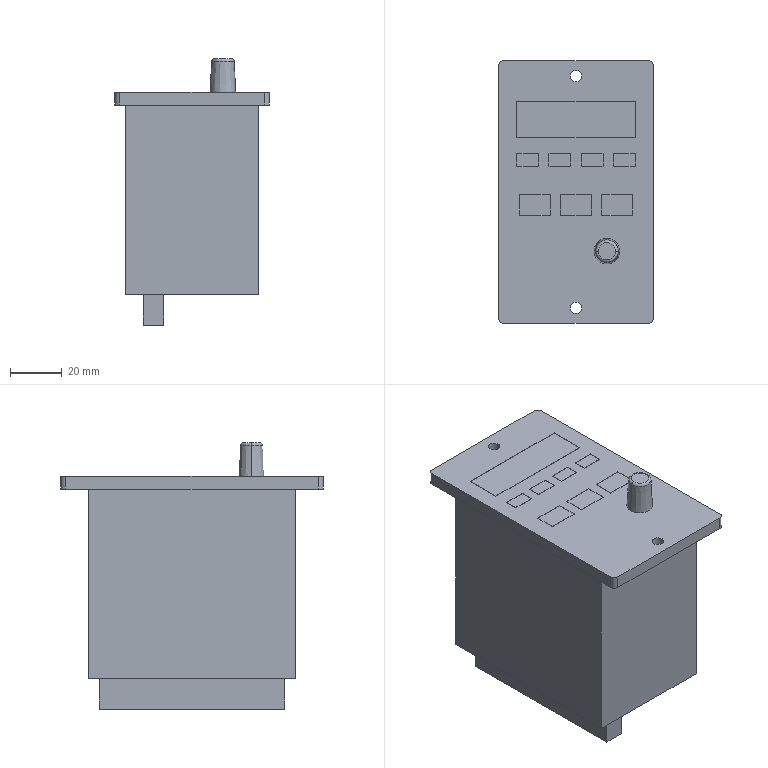Part | STEP file | SF06E_Default | 1 solid | 69 faces | box 60 x 102 x 103.5 mm | volume 343869 mm3 | plane 57 | cylinder 8 | torus 2 | cone 2 | commonest cylinder face diameters 4 x4 4.5 x4